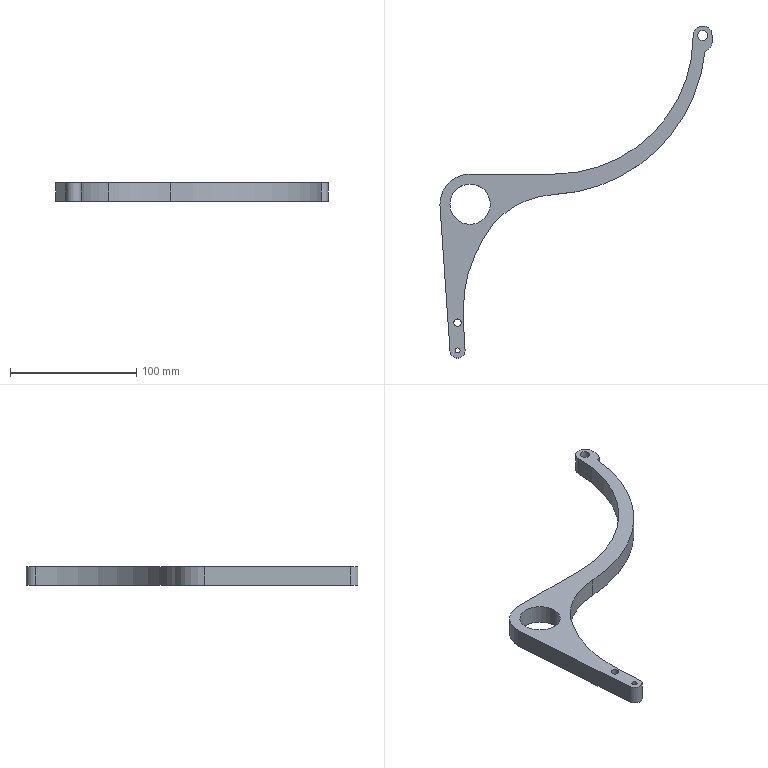Part | SolidWorks | features Extrusion 1 | 1 solid | 21 faces | box 216 x 263.5 x 15 mm | volume 92831 mm3 | cylinder 15 | plane 5 | spline 1 | commonest cylinder face diameters 4 x2 6 x2 7.838 x2 32 x2 12 x1 15 x1
STEP:
#1=CARTESIAN_POINT('',(-3.,22.,15.));
#2=VERTEX_POINT('',#1);
#3=CARTESIAN_POINT('',(3.,22.,15.));
#4=VERTEX_POINT('',#3);
#5=CARTESIAN_POINT('',(0.,22.,15.));
#6=DIRECTION('',(0.,0.,1.));
#7=DIRECTION('',(1.,0.,0.));
#8=AXIS2_PLACEMENT_3D('',#5,#6,#7);
#9=CIRCLE('',#8,3.);
#10=EDGE_CURVE('',#2,#4,#9,.T.);
#11=ORIENTED_EDGE('',*,*,#10,.T.);
#12=CARTESIAN_POINT('',(3.,22.,0.));
#13=VERTEX_POINT('',#12);
#14=CARTESIAN_POINT('',(3.,22.,15.));
#15=DIRECTION('',(0.,0.,-1.));
#16=VECTOR('',#15,1000.);
#17=LINE('',#14,#16);
#18=EDGE_CURVE('',#4,#13,#17,.T.);
#19=ORIENTED_EDGE('',*,*,#18,.T.);
#20=CARTESIAN_POINT('',(-3.,22.,0.));
#21=VERTEX_POINT('',#20);
#22=CARTESIAN_POINT('',(0.,22.,0.));
#23=DIRECTION('',(0.,0.,1.));
#24=DIRECTION('',(1.,0.,0.));
#25=AXIS2_PLACEMENT_3D('',#22,#23,#24);
#26=CIRCLE('',#25,3.);
#27=EDGE_CURVE('',#21,#13,#26,.T.);
#28=ORIENTED_EDGE('',*,*,#27,.F.);
#29=CARTESIAN_POINT('',(-3.,22.,15.));
#30=DIRECTION('',(0.,0.,-1.));
#31=VECTOR('',#30,1000.);
#32=LINE('',#29,#31);
#33=EDGE_CURVE('',#2,#21,#32,.T.);
#34=ORIENTED_EDGE('',*,*,#33,.F.);
#35=EDGE_LOOP('',(#11,#19,#28,#34));
#36=FACE_OUTER_BOUND('',#35,.T.);
#37=CARTESIAN_POINT('',(0.,22.,15.));
#38=DIRECTION('',(0.,0.,-1.));
#39=DIRECTION('',(-1.,0.,0.));
#40=AXIS2_PLACEMENT_3D('',#37,#38,#39);
#41=CYLINDRICAL_SURFACE('',#40,3.);
#42=ADVANCED_FACE('',(#36),#41,.F.);
#43=CARTESIAN_POINT('',(190.581,250.,15.));
#44=VERTEX_POINT('',#43);
#45=CARTESIAN_POINT('',(198.419,250.,15.));
#46=VERTEX_POINT('',#45);
#47=CARTESIAN_POINT('',(194.5,250.,15.));
#48=DIRECTION('',(0.,0.,1.));
#49=DIRECTION('',(1.,0.,0.));
#50=AXIS2_PLACEMENT_3D('',#47,#48,#49);
#51=CIRCLE('',#50,3.919);
#52=EDGE_CURVE('',#44,#46,#51,.T.);
#53=ORIENTED_EDGE('',*,*,#52,.T.);
#54=CARTESIAN_POINT('',(198.419,250.,0.));
#55=VERTEX_POINT('',#54);
#56=CARTESIAN_POINT('',(198.419,250.,15.));
#57=DIRECTION('',(0.,0.,-1.));
#58=VECTOR('',#57,1000.);
#59=LINE('',#56,#58);
#60=EDGE_CURVE('',#46,#55,#59,.T.);
#61=ORIENTED_EDGE('',*,*,#60,.T.);
#62=CARTESIAN_POINT('',(190.581,250.,0.));
#63=VERTEX_POINT('',#62);
#64=CARTESIAN_POINT('',(194.5,250.,0.));
#65=DIRECTION('',(0.,0.,1.));
#66=DIRECTION('',(1.,0.,0.));
#67=AXIS2_PLACEMENT_3D('',#64,#65,#66);
#68=CIRCLE('',#67,3.919);
#69=EDGE_CURVE('',#63,#55,#68,.T.);
#70=ORIENTED_EDGE('',*,*,#69,.F.);
#71=CARTESIAN_POINT('',(190.581,250.,15.));
#72=DIRECTION('',(0.,0.,-1.));
#73=VECTOR('',#72,1000.);
#74=LINE('',#71,#73);
#75=EDGE_CURVE('',#44,#63,#74,.T.);
#76=ORIENTED_EDGE('',*,*,#75,.F.);
#77=EDGE_LOOP('',(#53,#61,#70,#76));
#78=FACE_OUTER_BOUND('',#77,.T.);
#79=CARTESIAN_POINT('',(194.5,250.,15.));
#80=DIRECTION('',(0.,0.,-1.));
#81=DIRECTION('',(-1.,0.,0.));
#82=AXIS2_PLACEMENT_3D('',#79,#80,#81);
#83=CYLINDRICAL_SURFACE('',#82,3.919);
#84=ADVANCED_FACE('',(#78),#83,.F.);
#85=CARTESIAN_POINT('',(-6.,116.,15.));
#86=VERTEX_POINT('',#85);
#87=CARTESIAN_POINT('',(26.,116.,15.));
#88=VERTEX_POINT('',#87);
#89=CARTESIAN_POINT('',(10.,116.,15.));
#90=DIRECTION('',(0.,0.,1.));
#91=DIRECTION('',(1.,0.,0.));
#92=AXIS2_PLACEMENT_3D('',#89,#90,#91);
#93=CIRCLE('',#92,16.);
#94=EDGE_CURVE('',#86,#88,#93,.T.);
#95=ORIENTED_EDGE('',*,*,#94,.T.);
#96=CARTESIAN_POINT('',(26.,116.,0.));
#97=VERTEX_POINT('',#96);
#98=CARTESIAN_POINT('',(26.,116.,15.));
#99=DIRECTION('',(0.,0.,-1.));
#100=VECTOR('',#99,1000.);
#101=LINE('',#98,#100);
#102=EDGE_CURVE('',#88,#97,#101,.T.);
#103=ORIENTED_EDGE('',*,*,#102,.T.);
#104=CARTESIAN_POINT('',(-6.,116.,0.));
#105=VERTEX_POINT('',#104);
#106=CARTESIAN_POINT('',(10.,116.,0.));
#107=DIRECTION('',(0.,0.,1.));
#108=DIRECTION('',(1.,0.,0.));
#109=AXIS2_PLACEMENT_3D('',#106,#107,#108);
#110=CIRCLE('',#109,16.);
#111=EDGE_CURVE('',#105,#97,#110,.T.);
#112=ORIENTED_EDGE('',*,*,#111,.F.);
#113=CARTESIAN_POINT('',(-6.,116.,15.));
#114=DIRECTION('',(0.,0.,-1.));
#115=VECTOR('',#114,1000.);
#116=LINE('',#113,#115);
#117=EDGE_CURVE('',#86,#105,#116,.T.);
#118=ORIENTED_EDGE('',*,*,#117,.F.);
#119=EDGE_LOOP('',(#95,#103,#112,#118));
#120=FACE_OUTER_BOUND('',#119,.T.);
#121=CARTESIAN_POINT('',(10.,116.,15.));
#122=DIRECTION('',(0.,0.,-1.));
#123=DIRECTION('',(-1.,0.,0.));
#124=AXIS2_PLACEMENT_3D('',#121,#122,#123);
#125=CYLINDRICAL_SURFACE('',#124,16.);
#126=ADVANCED_FACE('',(#120),#125,.F.);
#127=CARTESIAN_POINT('',(-2.,0.,15.));
#128=VERTEX_POINT('',#127);
#129=CARTESIAN_POINT('',(2.,0.,15.));
#130=VERTEX_POINT('',#129);
#131=CARTESIAN_POINT('',(0.,0.,15.));
#132=DIRECTION('',(0.,0.,1.));
#133=DIRECTION('',(1.,0.,0.));
#134=AXIS2_PLACEMENT_3D('',#131,#132,#133);
#135=CIRCLE('',#134,2.);
#136=EDGE_CURVE('',#128,#130,#135,.T.);
#137=ORIENTED_EDGE('',*,*,#136,.T.);
#138=CARTESIAN_POINT('',(2.,0.,0.));
#139=VERTEX_POINT('',#138);
#140=CARTESIAN_POINT('',(2.,0.,15.));
#141=DIRECTION('',(0.,0.,-1.));
#142=VECTOR('',#141,1000.);
#143=LINE('',#140,#142);
#144=EDGE_CURVE('',#130,#139,#143,.T.);
#145=ORIENTED_EDGE('',*,*,#144,.T.);
#146=CARTESIAN_POINT('',(-2.,0.,0.));
#147=VERTEX_POINT('',#146);
#148=CARTESIAN_POINT('',(0.,0.,0.));
#149=DIRECTION('',(0.,0.,1.));
#150=DIRECTION('',(1.,0.,0.));
#151=AXIS2_PLACEMENT_3D('',#148,#149,#150);
#152=CIRCLE('',#151,2.);
#153=EDGE_CURVE('',#147,#139,#152,.T.);
#154=ORIENTED_EDGE('',*,*,#153,.F.);
#155=CARTESIAN_POINT('',(-2.,0.,15.));
#156=DIRECTION('',(0.,0.,-1.));
#157=VECTOR('',#156,1000.);
#158=LINE('',#155,#157);
#159=EDGE_CURVE('',#128,#147,#158,.T.);
#160=ORIENTED_EDGE('',*,*,#159,.F.);
#161=EDGE_LOOP('',(#137,#145,#154,#160));
#162=FACE_OUTER_BOUND('',#161,.T.);
#163=CARTESIAN_POINT('',(0.,0.,15.));
#164=DIRECTION('',(0.,0.,-1.));
#165=DIRECTION('',(-1.,0.,0.));
#166=AXIS2_PLACEMENT_3D('',#163,#164,#165);
#167=CYLINDRICAL_SURFACE('',#166,2.);
#168=ADVANCED_FACE('',(#162),#167,.F.);
#169=ORIENTED_EDGE('',*,*,#52,.F.);
#170=CARTESIAN_POINT('',(194.5,250.,15.));
#171=DIRECTION('',(0.,0.,1.));
#172=DIRECTION('',(1.,0.,0.));
#173=AXIS2_PLACEMENT_3D('',#170,#171,#172);
#174=CIRCLE('',#173,3.919);
#175=EDGE_CURVE('',#46,#44,#174,.T.);
#176=ORIENTED_EDGE('',*,*,#175,.F.);
#177=EDGE_LOOP('',(#169,#176));
#178=FACE_BOUND('',#177,.T.);
#179=ORIENTED_EDGE('',*,*,#136,.F.);
#180=CARTESIAN_POINT('',(0.,0.,15.));
#181=DIRECTION('',(0.,0.,1.));
#182=DIRECTION('',(1.,0.,0.));
#183=AXIS2_PLACEMENT_3D('',#180,#181,#182);
#184=CIRCLE('',#183,2.);
#185=EDGE_CURVE('',#130,#128,#184,.T.);
#186=ORIENTED_EDGE('',*,*,#185,.F.);
#187=EDGE_LOOP('',(#179,#186));
#188=FACE_BOUND('',#187,.T.);
#189=CARTESIAN_POINT('',(10.,140.,15.));
#190=VERTEX_POINT('',#189);
#191=CARTESIAN_POINT('',(-14.,116.,15.));
#192=VERTEX_POINT('',#191);
#193=CARTESIAN_POINT('',(10.,116.,15.));
#194=DIRECTION('',(0.,0.,1.));
#195=DIRECTION('',(1.,0.,0.));
#196=AXIS2_PLACEMENT_3D('',#193,#194,#195);
#197=CIRCLE('',#196,24.);
#198=EDGE_CURVE('',#190,#192,#197,.T.);
#199=ORIENTED_EDGE('',*,*,#198,.T.);
#200=CARTESIAN_POINT('',(-6.,0.,15.));
#201=VERTEX_POINT('',#200);
#202=CARTESIAN_POINT('',(-14.,116.,15.));
#203=DIRECTION('',(0.0688,-0.9976,0.));
#204=VECTOR('',#203,1000.);
#205=LINE('',#202,#204);
#206=EDGE_CURVE('',#192,#201,#205,.T.);
#207=ORIENTED_EDGE('',*,*,#206,.T.);
#208=CARTESIAN_POINT('',(6.,0.,15.));
#209=VERTEX_POINT('',#208);
#210=CARTESIAN_POINT('',(0.,0.,15.));
#211=DIRECTION('',(0.,0.,1.));
#212=DIRECTION('',(1.,0.,0.));
#213=AXIS2_PLACEMENT_3D('',#210,#211,#212);
#214=CIRCLE('',#213,6.);
#215=EDGE_CURVE('',#201,#209,#214,.T.);
#216=ORIENTED_EDGE('',*,*,#215,.T.);
#217=CARTESIAN_POINT('',(28.005,100.131,15.));
#218=VERTEX_POINT('',#217);
#219=CARTESIAN_POINT('',(6.,0.,15.));
#220=CARTESIAN_POINT('',(1.589,45.681,15.));
#221=CARTESIAN_POINT('',(5.604,67.643,15.));
#222=CARTESIAN_POINT('',(28.005,100.131,15.));
#223=B_SPLINE_CURVE_WITH_KNOTS('',3,(#219,#220,#221,#222),.UNSPECIFIED.,.F.,.F.,(4,4),(0.,0.7882),.UNSPECIFIED.);
#224=EDGE_CURVE('',#209,#218,#223,.T.);
#225=ORIENTED_EDGE('',*,*,#224,.T.);
#226=CARTESIAN_POINT('',(77.,123.767,15.));
#227=VERTEX_POINT('',#226);
#228=CARTESIAN_POINT('',(80.543,53.825,15.));
#229=DIRECTION('',(0.,0.,-1.));
#230=DIRECTION('',(1.,0.,0.));
#231=AXIS2_PLACEMENT_3D('',#228,#229,#230);
#232=CIRCLE('',#231,70.032);
#233=EDGE_CURVE('',#218,#227,#232,.T.);
#234=ORIENTED_EDGE('',*,*,#233,.T.);
#235=CARTESIAN_POINT('',(196.38,237.495,15.));
#236=VERTEX_POINT('',#235);
#237=CARTESIAN_POINT('',(70.606,250.,15.));
#238=DIRECTION('',(0.,0.,1.));
#239=DIRECTION('',(1.,0.,0.));
#240=AXIS2_PLACEMENT_3D('',#237,#238,#239);
#241=CIRCLE('',#240,126.394);
#242=EDGE_CURVE('',#227,#236,#241,.T.);
#243=ORIENTED_EDGE('',*,*,#242,.T.);
#244=CARTESIAN_POINT('',(202.,245.,15.));
#245=VERTEX_POINT('',#244);
#246=CARTESIAN_POINT('',(194.179,245.,15.));
#247=DIRECTION('',(0.,0.,1.));
#248=DIRECTION('',(1.,0.,0.));
#249=AXIS2_PLACEMENT_3D('',#246,#247,#248);
#250=CIRCLE('',#249,7.821);
#251=EDGE_CURVE('',#236,#245,#250,.T.);
#252=ORIENTED_EDGE('',*,*,#251,.T.);
#253=CARTESIAN_POINT('',(202.,250.,15.));
#254=VERTEX_POINT('',#253);
#255=CARTESIAN_POINT('',(202.,250.,15.));
#256=DIRECTION('',(0.,1.,0.));
#257=VECTOR('',#256,1000.);
#258=LINE('',#255,#257);
#259=EDGE_CURVE('',#245,#254,#258,.T.);
#260=ORIENTED_EDGE('',*,*,#259,.T.);
#261=CARTESIAN_POINT('',(187.,250.,15.));
#262=VERTEX_POINT('',#261);
#263=CARTESIAN_POINT('',(194.5,250.,15.));
#264=DIRECTION('',(0.,0.,1.));
#265=DIRECTION('',(1.,0.,0.));
#266=AXIS2_PLACEMENT_3D('',#263,#264,#265);
#267=CIRCLE('',#266,7.5);
#268=EDGE_CURVE('',#254,#262,#267,.T.);
#269=ORIENTED_EDGE('',*,*,#268,.T.);
#270=CARTESIAN_POINT('',(77.,140.,15.));
#271=VERTEX_POINT('',#270);
#272=CARTESIAN_POINT('',(77.,250.,15.));
#273=DIRECTION('',(0.,0.,-1.));
#274=DIRECTION('',(1.,0.,0.));
#275=AXIS2_PLACEMENT_3D('',#272,#273,#274);
#276=CIRCLE('',#275,110.);
#277=EDGE_CURVE('',#262,#271,#276,.T.);
#278=ORIENTED_EDGE('',*,*,#277,.T.);
#279=CARTESIAN_POINT('',(10.,140.,15.));
#280=DIRECTION('',(-1.,0.,0.));
#281=VECTOR('',#280,1000.);
#282=LINE('',#279,#281);
#283=EDGE_CURVE('',#271,#190,#282,.T.);
#284=ORIENTED_EDGE('',*,*,#283,.T.);
#285=EDGE_LOOP('',(#199,#207,#216,#225,#234,#243,#252,#260,#269,#278,#284));
#286=FACE_OUTER_BOUND('',#285,.T.);
#287=ORIENTED_EDGE('',*,*,#94,.F.);
#288=CARTESIAN_POINT('',(10.,116.,15.));
#289=DIRECTION('',(0.,0.,1.));
#290=DIRECTION('',(1.,0.,0.));
#291=AXIS2_PLACEMENT_3D('',#288,#289,#290);
#292=CIRCLE('',#291,16.);
#293=EDGE_CURVE('',#88,#86,#292,.T.);
#294=ORIENTED_EDGE('',*,*,#293,.F.);
#295=EDGE_LOOP('',(#287,#294));
#296=FACE_BOUND('',#295,.T.);
#297=ORIENTED_EDGE('',*,*,#10,.F.);
#298=CARTESIAN_POINT('',(0.,22.,15.));
#299=DIRECTION('',(0.,0.,1.));
#300=DIRECTION('',(1.,0.,0.));
#301=AXIS2_PLACEMENT_3D('',#298,#299,#300);
#302=CIRCLE('',#301,3.);
#303=EDGE_CURVE('',#4,#2,#302,.T.);
#304=ORIENTED_EDGE('',*,*,#303,.F.);
#305=EDGE_LOOP('',(#297,#304));
#306=FACE_BOUND('',#305,.T.);
#307=CARTESIAN_POINT('',(10.,116.,15.));
#308=DIRECTION('',(0.,0.,1.));
#309=DIRECTION('',(1.,0.,0.));
#310=AXIS2_PLACEMENT_3D('',#307,#308,#309);
#311=PLANE('',#310);
#312=ADVANCED_FACE('',(#178,#188,#286,#296,#306),#311,.T.);
#313=CARTESIAN_POINT('',(10.,140.,0.));
#314=VERTEX_POINT('',#313);
#315=CARTESIAN_POINT('',(-14.,116.,0.));
#316=VERTEX_POINT('',#315);
#317=CARTESIAN_POINT('',(10.,116.,0.));
#318=DIRECTION('',(0.,0.,1.));
#319=DIRECTION('',(1.,0.,0.));
#320=AXIS2_PLACEMENT_3D('',#317,#318,#319);
#321=CIRCLE('',#320,24.);
#322=EDGE_CURVE('',#314,#316,#321,.T.);
#323=ORIENTED_EDGE('',*,*,#322,.F.);
#324=CARTESIAN_POINT('',(77.,140.,0.));
#325=VERTEX_POINT('',#324);
#326=CARTESIAN_POINT('',(10.,140.,0.));
#327=DIRECTION('',(-1.,0.,0.));
#328=VECTOR('',#327,1000.);
#329=LINE('',#326,#328);
#330=EDGE_CURVE('',#325,#314,#329,.T.);
#331=ORIENTED_EDGE('',*,*,#330,.F.);
#332=CARTESIAN_POINT('',(187.,250.,0.));
#333=VERTEX_POINT('',#332);
#334=CARTESIAN_POINT('',(77.,250.,0.));
#335=DIRECTION('',(0.,0.,-1.));
#336=DIRECTION('',(1.,0.,0.));
#337=AXIS2_PLACEMENT_3D('',#334,#335,#336);
#338=CIRCLE('',#337,110.);
#339=EDGE_CURVE('',#333,#325,#338,.T.);
#340=ORIENTED_EDGE('',*,*,#339,.F.);
#341=CARTESIAN_POINT('',(202.,250.,0.));
#342=VERTEX_POINT('',#341);
#343=CARTESIAN_POINT('',(194.5,250.,0.));
#344=DIRECTION('',(0.,0.,1.));
#345=DIRECTION('',(1.,0.,0.));
#346=AXIS2_PLACEMENT_3D('',#343,#344,#345);
#347=CIRCLE('',#346,7.5);
#348=EDGE_CURVE('',#342,#333,#347,.T.);
#349=ORIENTED_EDGE('',*,*,#348,.F.);
#350=CARTESIAN_POINT('',(202.,245.,0.));
#351=VERTEX_POINT('',#350);
#352=CARTESIAN_POINT('',(202.,250.,0.));
#353=DIRECTION('',(0.,1.,0.));
#354=VECTOR('',#353,1000.);
#355=LINE('',#352,#354);
#356=EDGE_CURVE('',#351,#342,#355,.T.);
#357=ORIENTED_EDGE('',*,*,#356,.F.);
#358=CARTESIAN_POINT('',(196.38,237.495,0.));
#359=VERTEX_POINT('',#358);
#360=CARTESIAN_POINT('',(194.179,245.,0.));
#361=DIRECTION('',(0.,0.,1.));
#362=DIRECTION('',(1.,0.,0.));
#363=AXIS2_PLACEMENT_3D('',#360,#361,#362);
#364=CIRCLE('',#363,7.821);
#365=EDGE_CURVE('',#359,#351,#364,.T.);
#366=ORIENTED_EDGE('',*,*,#365,.F.);
#367=CARTESIAN_POINT('',(77.,123.767,0.));
#368=VERTEX_POINT('',#367);
#369=CARTESIAN_POINT('',(70.606,250.,0.));
#370=DIRECTION('',(0.,0.,1.));
#371=DIRECTION('',(1.,0.,0.));
#372=AXIS2_PLACEMENT_3D('',#369,#370,#371);
#373=CIRCLE('',#372,126.394);
#374=EDGE_CURVE('',#368,#359,#373,.T.);
#375=ORIENTED_EDGE('',*,*,#374,.F.);
#376=CARTESIAN_POINT('',(28.005,100.131,0.));
#377=VERTEX_POINT('',#376);
#378=CARTESIAN_POINT('',(80.543,53.825,0.));
#379=DIRECTION('',(0.,0.,-1.));
#380=DIRECTION('',(1.,0.,0.));
#381=AXIS2_PLACEMENT_3D('',#378,#379,#380);
#382=CIRCLE('',#381,70.032);
#383=EDGE_CURVE('',#377,#368,#382,.T.);
#384=ORIENTED_EDGE('',*,*,#383,.F.);
#385=CARTESIAN_POINT('',(6.,0.,0.));
#386=VERTEX_POINT('',#385);
#387=CARTESIAN_POINT('',(6.,0.,0.));
#388=CARTESIAN_POINT('',(1.589,45.681,0.));
#389=CARTESIAN_POINT('',(5.604,67.643,0.));
#390=CARTESIAN_POINT('',(28.005,100.131,0.));
#391=B_SPLINE_CURVE_WITH_KNOTS('',3,(#387,#388,#389,#390),.UNSPECIFIED.,.F.,.F.,(4,4),(0.,0.7882),.UNSPECIFIED.);
#392=EDGE_CURVE('',#386,#377,#391,.T.);
#393=ORIENTED_EDGE('',*,*,#392,.F.);
#394=CARTESIAN_POINT('',(-6.,0.,0.));
#395=VERTEX_POINT('',#394);
#396=CARTESIAN_POINT('',(0.,0.,0.));
#397=DIRECTION('',(0.,0.,1.));
#398=DIRECTION('',(1.,0.,0.));
#399=AXIS2_PLACEMENT_3D('',#396,#397,#398);
#400=CIRCLE('',#399,6.);
#401=EDGE_CURVE('',#395,#386,#400,.T.);
#402=ORIENTED_EDGE('',*,*,#401,.F.);
#403=CARTESIAN_POINT('',(-14.,116.,0.));
#404=DIRECTION('',(0.0688,-0.9976,0.));
#405=VECTOR('',#404,1000.);
#406=LINE('',#403,#405);
#407=EDGE_CURVE('',#316,#395,#406,.T.);
#408=ORIENTED_EDGE('',*,*,#407,.F.);
#409=EDGE_LOOP('',(#323,#331,#340,#349,#357,#366,#375,#384,#393,#402,#408));
#410=FACE_OUTER_BOUND('',#409,.T.);
#411=ORIENTED_EDGE('',*,*,#153,.T.);
#412=CARTESIAN_POINT('',(0.,0.,0.));
#413=DIRECTION('',(0.,0.,1.));
#414=DIRECTION('',(1.,0.,0.));
#415=AXIS2_PLACEMENT_3D('',#412,#413,#414);
#416=CIRCLE('',#415,2.);
#417=EDGE_CURVE('',#139,#147,#416,.T.);
#418=ORIENTED_EDGE('',*,*,#417,.T.);
#419=EDGE_LOOP('',(#411,#418));
#420=FACE_BOUND('',#419,.T.);
#421=ORIENTED_EDGE('',*,*,#111,.T.);
#422=CARTESIAN_POINT('',(10.,116.,0.));
#423=DIRECTION('',(0.,0.,1.));
#424=DIRECTION('',(1.,0.,0.));
#425=AXIS2_PLACEMENT_3D('',#422,#423,#424);
#426=CIRCLE('',#425,16.);
#427=EDGE_CURVE('',#97,#105,#426,.T.);
#428=ORIENTED_EDGE('',*,*,#427,.T.);
#429=EDGE_LOOP('',(#421,#428));
#430=FACE_BOUND('',#429,.T.);
#431=ORIENTED_EDGE('',*,*,#69,.T.);
#432=CARTESIAN_POINT('',(194.5,250.,0.));
#433=DIRECTION('',(0.,0.,1.));
#434=DIRECTION('',(1.,0.,0.));
#435=AXIS2_PLACEMENT_3D('',#432,#433,#434);
#436=CIRCLE('',#435,3.919);
#437=EDGE_CURVE('',#55,#63,#436,.T.);
#438=ORIENTED_EDGE('',*,*,#437,.T.);
#439=EDGE_LOOP('',(#431,#438));
#440=FACE_BOUND('',#439,.T.);
#441=ORIENTED_EDGE('',*,*,#27,.T.);
#442=CARTESIAN_POINT('',(0.,22.,0.));
#443=DIRECTION('',(0.,0.,1.));
#444=DIRECTION('',(1.,0.,0.));
#445=AXIS2_PLACEMENT_3D('',#442,#443,#444);
#446=CIRCLE('',#445,3.);
#447=EDGE_CURVE('',#13,#21,#446,.T.);
#448=ORIENTED_EDGE('',*,*,#447,.T.);
#449=EDGE_LOOP('',(#441,#448));
#450=FACE_BOUND('',#449,.T.);
#451=CARTESIAN_POINT('',(10.,116.,0.));
#452=DIRECTION('',(0.,0.,1.));
#453=DIRECTION('',(1.,0.,0.));
#454=AXIS2_PLACEMENT_3D('',#451,#452,#453);
#455=PLANE('',#454);
#456=ADVANCED_FACE('',(#410,#420,#430,#440,#450),#455,.F.);
#457=ORIENTED_EDGE('',*,*,#322,.T.);
#458=CARTESIAN_POINT('',(-14.,116.,15.));
#459=DIRECTION('',(0.,0.,-1.));
#460=VECTOR('',#459,1000.);
#461=LINE('',#458,#460);
#462=EDGE_CURVE('',#192,#316,#461,.T.);
#463=ORIENTED_EDGE('',*,*,#462,.F.);
#464=ORIENTED_EDGE('',*,*,#198,.F.);
#465=CARTESIAN_POINT('',(10.,140.,15.));
#466=DIRECTION('',(0.,0.,-1.));
#467=VECTOR('',#466,1000.);
#468=LINE('',#465,#467);
#469=EDGE_CURVE('',#190,#314,#468,.T.);
#470=ORIENTED_EDGE('',*,*,#469,.T.);
#471=EDGE_LOOP('',(#457,#463,#464,#470));
#472=FACE_OUTER_BOUND('',#471,.T.);
#473=CARTESIAN_POINT('',(10.,116.,15.));
#474=DIRECTION('',(0.,0.,-1.));
#475=DIRECTION('',(-1.,0.,0.));
#476=AXIS2_PLACEMENT_3D('',#473,#474,#475);
#477=CYLINDRICAL_SURFACE('',#476,24.);
#478=ADVANCED_FACE('',(#472),#477,.T.);
#479=ORIENTED_EDGE('',*,*,#407,.T.);
#480=CARTESIAN_POINT('',(-6.,0.,15.));
#481=DIRECTION('',(0.,0.,-1.));
#482=VECTOR('',#481,1000.);
#483=LINE('',#480,#482);
#484=EDGE_CURVE('',#201,#395,#483,.T.);
#485=ORIENTED_EDGE('',*,*,#484,.F.);
#486=ORIENTED_EDGE('',*,*,#206,.F.);
#487=ORIENTED_EDGE('',*,*,#462,.T.);
#488=EDGE_LOOP('',(#479,#485,#486,#487));
#489=FACE_OUTER_BOUND('',#488,.T.);
#490=CARTESIAN_POINT('',(-14.,116.,15.));
#491=DIRECTION('',(0.9976,0.0688,0.));
#492=DIRECTION('',(-0.0688,0.9976,0.));
#493=AXIS2_PLACEMENT_3D('',#490,#491,#492);
#494=PLANE('',#493);
#495=ADVANCED_FACE('',(#489),#494,.F.);
#496=ORIENTED_EDGE('',*,*,#401,.T.);
#497=CARTESIAN_POINT('',(6.,0.,15.));
#498=DIRECTION('',(0.,0.,-1.));
#499=VECTOR('',#498,1000.);
#500=LINE('',#497,#499);
#501=EDGE_CURVE('',#209,#386,#500,.T.);
#502=ORIENTED_EDGE('',*,*,#501,.F.);
#503=ORIENTED_EDGE('',*,*,#215,.F.);
#504=ORIENTED_EDGE('',*,*,#484,.T.);
#505=EDGE_LOOP('',(#496,#502,#503,#504));
#506=FACE_OUTER_BOUND('',#505,.T.);
#507=CARTESIAN_POINT('',(0.,0.,15.));
#508=DIRECTION('',(0.,0.,-1.));
#509=DIRECTION('',(-1.,0.,0.));
#510=AXIS2_PLACEMENT_3D('',#507,#508,#509);
#511=CYLINDRICAL_SURFACE('',#510,6.);
#512=ADVANCED_FACE('',(#506),#511,.T.);
#513=ORIENTED_EDGE('',*,*,#392,.T.);
#514=CARTESIAN_POINT('',(28.005,100.131,15.));
#515=DIRECTION('',(0.,0.,-1.));
#516=VECTOR('',#515,1000.);
#517=LINE('',#514,#516);
#518=EDGE_CURVE('',#218,#377,#517,.T.);
#519=ORIENTED_EDGE('',*,*,#518,.F.);
#520=ORIENTED_EDGE('',*,*,#224,.F.);
#521=ORIENTED_EDGE('',*,*,#501,.T.);
#522=EDGE_LOOP('',(#513,#519,#520,#521));
#523=FACE_OUTER_BOUND('',#522,.T.);
#524=CARTESIAN_POINT('',(6.,0.,15.));
#525=CARTESIAN_POINT('',(6.,0.,0.));
#526=CARTESIAN_POINT('',(1.589,45.681,15.));
#527=CARTESIAN_POINT('',(1.589,45.681,0.));
#528=CARTESIAN_POINT('',(5.604,67.643,15.));
#529=CARTESIAN_POINT('',(5.604,67.643,0.));
#530=CARTESIAN_POINT('',(28.005,100.131,15.));
#531=CARTESIAN_POINT('',(28.005,100.131,0.));
#532=B_SPLINE_SURFACE_WITH_KNOTS('',3,1,((#524,#525),(#526,#527),(#528,#529),(#530,#531)),.UNSPECIFIED.,.F.,.F.,.F.,(4,4),(2,2),(0.,0.7882),(0.,1.),.UNSPECIFIED.);
#533=ADVANCED_FACE('',(#523),#532,.F.);
#534=ORIENTED_EDGE('',*,*,#383,.T.);
#535=CARTESIAN_POINT('',(77.,123.767,15.));
#536=DIRECTION('',(0.,0.,-1.));
#537=VECTOR('',#536,1000.);
#538=LINE('',#535,#537);
#539=EDGE_CURVE('',#227,#368,#538,.T.);
#540=ORIENTED_EDGE('',*,*,#539,.F.);
#541=ORIENTED_EDGE('',*,*,#233,.F.);
#542=ORIENTED_EDGE('',*,*,#518,.T.);
#543=EDGE_LOOP('',(#534,#540,#541,#542));
#544=FACE_OUTER_BOUND('',#543,.T.);
#545=CARTESIAN_POINT('',(80.543,53.825,15.));
#546=DIRECTION('',(0.,0.,-1.));
#547=DIRECTION('',(-1.,0.,0.));
#548=AXIS2_PLACEMENT_3D('',#545,#546,#547);
#549=CYLINDRICAL_SURFACE('',#548,70.032);
#550=ADVANCED_FACE('',(#544),#549,.F.);
#551=ORIENTED_EDGE('',*,*,#374,.T.);
#552=CARTESIAN_POINT('',(196.38,237.495,15.));
#553=DIRECTION('',(0.,0.,-1.));
#554=VECTOR('',#553,1000.);
#555=LINE('',#552,#554);
#556=EDGE_CURVE('',#236,#359,#555,.T.);
#557=ORIENTED_EDGE('',*,*,#556,.F.);
#558=ORIENTED_EDGE('',*,*,#242,.F.);
#559=ORIENTED_EDGE('',*,*,#539,.T.);
#560=EDGE_LOOP('',(#551,#557,#558,#559));
#561=FACE_OUTER_BOUND('',#560,.T.);
#562=CARTESIAN_POINT('',(70.606,250.,15.));
#563=DIRECTION('',(0.,0.,-1.));
#564=DIRECTION('',(-1.,0.,0.));
#565=AXIS2_PLACEMENT_3D('',#562,#563,#564);
#566=CYLINDRICAL_SURFACE('',#565,126.394);
#567=ADVANCED_FACE('',(#561),#566,.T.);
#568=ORIENTED_EDGE('',*,*,#365,.T.);
#569=CARTESIAN_POINT('',(202.,245.,15.));
#570=DIRECTION('',(0.,0.,-1.));
#571=VECTOR('',#570,1000.);
#572=LINE('',#569,#571);
#573=EDGE_CURVE('',#245,#351,#572,.T.);
#574=ORIENTED_EDGE('',*,*,#573,.F.);
#575=ORIENTED_EDGE('',*,*,#251,.F.);
#576=ORIENTED_EDGE('',*,*,#556,.T.);
#577=EDGE_LOOP('',(#568,#574,#575,#576));
#578=FACE_OUTER_BOUND('',#577,.T.);
#579=CARTESIAN_POINT('',(194.179,245.,15.));
#580=DIRECTION('',(0.,0.,-1.));
#581=DIRECTION('',(-1.,0.,0.));
#582=AXIS2_PLACEMENT_3D('',#579,#580,#581);
#583=CYLINDRICAL_SURFACE('',#582,7.821);
#584=ADVANCED_FACE('',(#578),#583,.T.);
#585=ORIENTED_EDGE('',*,*,#356,.T.);
#586=CARTESIAN_POINT('',(202.,250.,15.));
#587=DIRECTION('',(0.,0.,-1.));
#588=VECTOR('',#587,1000.);
#589=LINE('',#586,#588);
#590=EDGE_CURVE('',#254,#342,#589,.T.);
#591=ORIENTED_EDGE('',*,*,#590,.F.);
#592=ORIENTED_EDGE('',*,*,#259,.F.);
#593=ORIENTED_EDGE('',*,*,#573,.T.);
#594=EDGE_LOOP('',(#585,#591,#592,#593));
#595=FACE_OUTER_BOUND('',#594,.T.);
#596=CARTESIAN_POINT('',(202.,250.,15.));
#597=DIRECTION('',(-1.,0.,0.));
#598=DIRECTION('',(0.,0.,1.));
#599=AXIS2_PLACEMENT_3D('',#596,#597,#598);
#600=PLANE('',#599);
#601=ADVANCED_FACE('',(#595),#600,.F.);
#602=ORIENTED_EDGE('',*,*,#348,.T.);
#603=CARTESIAN_POINT('',(187.,250.,15.));
#604=DIRECTION('',(0.,0.,-1.));
#605=VECTOR('',#604,1000.);
#606=LINE('',#603,#605);
#607=EDGE_CURVE('',#262,#333,#606,.T.);
#608=ORIENTED_EDGE('',*,*,#607,.F.);
#609=ORIENTED_EDGE('',*,*,#268,.F.);
#610=ORIENTED_EDGE('',*,*,#590,.T.);
#611=EDGE_LOOP('',(#602,#608,#609,#610));
#612=FACE_OUTER_BOUND('',#611,.T.);
#613=CARTESIAN_POINT('',(194.5,250.,15.));
#614=DIRECTION('',(0.,0.,-1.));
#615=DIRECTION('',(-1.,0.,0.));
#616=AXIS2_PLACEMENT_3D('',#613,#614,#615);
#617=CYLINDRICAL_SURFACE('',#616,7.5);
#618=ADVANCED_FACE('',(#612),#617,.T.);
#619=ORIENTED_EDGE('',*,*,#339,.T.);
#620=CARTESIAN_POINT('',(77.,140.,15.));
#621=DIRECTION('',(0.,0.,-1.));
#622=VECTOR('',#621,1000.);
#623=LINE('',#620,#622);
#624=EDGE_CURVE('',#271,#325,#623,.T.);
#625=ORIENTED_EDGE('',*,*,#624,.F.);
#626=ORIENTED_EDGE('',*,*,#277,.F.);
#627=ORIENTED_EDGE('',*,*,#607,.T.);
#628=EDGE_LOOP('',(#619,#625,#626,#627));
#629=FACE_OUTER_BOUND('',#628,.T.);
#630=CARTESIAN_POINT('',(77.,250.,15.));
#631=DIRECTION('',(0.,0.,-1.));
#632=DIRECTION('',(-1.,0.,0.));
#633=AXIS2_PLACEMENT_3D('',#630,#631,#632);
#634=CYLINDRICAL_SURFACE('',#633,110.);
#635=ADVANCED_FACE('',(#629),#634,.F.);
#636=ORIENTED_EDGE('',*,*,#330,.T.);
#637=ORIENTED_EDGE('',*,*,#469,.F.);
#638=ORIENTED_EDGE('',*,*,#283,.F.);
#639=ORIENTED_EDGE('',*,*,#624,.T.);
#640=EDGE_LOOP('',(#636,#637,#638,#639));
#641=FACE_OUTER_BOUND('',#640,.T.);
#642=CARTESIAN_POINT('',(10.,140.,15.));
#643=DIRECTION('',(0.,-1.,0.));
#644=DIRECTION('',(0.,0.,-1.));
#645=AXIS2_PLACEMENT_3D('',#642,#643,#644);
#646=PLANE('',#645);
#647=ADVANCED_FACE('',(#641),#646,.F.);
#648=ORIENTED_EDGE('',*,*,#144,.F.);
#649=ORIENTED_EDGE('',*,*,#185,.T.);
#650=ORIENTED_EDGE('',*,*,#159,.T.);
#651=ORIENTED_EDGE('',*,*,#417,.F.);
#652=EDGE_LOOP('',(#648,#649,#650,#651));
#653=FACE_OUTER_BOUND('',#652,.T.);
#654=CARTESIAN_POINT('',(0.,0.,15.));
#655=DIRECTION('',(0.,0.,-1.));
#656=DIRECTION('',(-1.,0.,0.));
#657=AXIS2_PLACEMENT_3D('',#654,#655,#656);
#658=CYLINDRICAL_SURFACE('',#657,2.);
#659=ADVANCED_FACE('',(#653),#658,.F.);
#660=ORIENTED_EDGE('',*,*,#102,.F.);
#661=ORIENTED_EDGE('',*,*,#293,.T.);
#662=ORIENTED_EDGE('',*,*,#117,.T.);
#663=ORIENTED_EDGE('',*,*,#427,.F.);
#664=EDGE_LOOP('',(#660,#661,#662,#663));
#665=FACE_OUTER_BOUND('',#664,.T.);
#666=CARTESIAN_POINT('',(10.,116.,15.));
#667=DIRECTION('',(0.,0.,-1.));
#668=DIRECTION('',(-1.,0.,0.));
#669=AXIS2_PLACEMENT_3D('',#666,#667,#668);
#670=CYLINDRICAL_SURFACE('',#669,16.);
#671=ADVANCED_FACE('',(#665),#670,.F.);
#672=ORIENTED_EDGE('',*,*,#60,.F.);
#673=ORIENTED_EDGE('',*,*,#175,.T.);
#674=ORIENTED_EDGE('',*,*,#75,.T.);
#675=ORIENTED_EDGE('',*,*,#437,.F.);
#676=EDGE_LOOP('',(#672,#673,#674,#675));
#677=FACE_OUTER_BOUND('',#676,.T.);
#678=CARTESIAN_POINT('',(194.5,250.,15.));
#679=DIRECTION('',(0.,0.,-1.));
#680=DIRECTION('',(-1.,0.,0.));
#681=AXIS2_PLACEMENT_3D('',#678,#679,#680);
#682=CYLINDRICAL_SURFACE('',#681,3.919);
#683=ADVANCED_FACE('',(#677),#682,.F.);
#684=ORIENTED_EDGE('',*,*,#18,.F.);
#685=ORIENTED_EDGE('',*,*,#303,.T.);
#686=ORIENTED_EDGE('',*,*,#33,.T.);
#687=ORIENTED_EDGE('',*,*,#447,.F.);
#688=EDGE_LOOP('',(#684,#685,#686,#687));
#689=FACE_OUTER_BOUND('',#688,.T.);
#690=CARTESIAN_POINT('',(0.,22.,15.));
#691=DIRECTION('',(0.,0.,-1.));
#692=DIRECTION('',(-1.,0.,0.));
#693=AXIS2_PLACEMENT_3D('',#690,#691,#692);
#694=CYLINDRICAL_SURFACE('',#693,3.);
#695=ADVANCED_FACE('',(#689),#694,.F.);
#696=CLOSED_SHELL('',(#42,#84,#126,#168,#312,#456,#478,#495,#512,#533,#550,#567,#584,#601,#618,#635,#647,#659,#671,#683,#695));
#697=MANIFOLD_SOLID_BREP('',#696);
#698=CARTESIAN_POINT('',(0.,0.,0.));
#699=DIRECTION('',(0.,0.,1.));
#700=DIRECTION('',(1.,0.,0.));
#701=AXIS2_PLACEMENT_3D('',#698,#699,#700);
#702=(LENGTH_UNIT()NAMED_UNIT(*)SI_UNIT(.MILLI.,.METRE.));
#703=UNCERTAINTY_MEASURE_WITH_UNIT(LENGTH_MEASURE(0.00001),#702,'','');
#704=(NAMED_UNIT(*)PLANE_ANGLE_UNIT()SI_UNIT($,.RADIAN.));
#705=(NAMED_UNIT(*)SI_UNIT($,.STERADIAN.)SOLID_ANGLE_UNIT());
#706=(GEOMETRIC_REPRESENTATION_CONTEXT(3)GLOBAL_UNCERTAINTY_ASSIGNED_CONTEXT((#703))GLOBAL_UNIT_ASSIGNED_CONTEXT((#702,#704,#705))REPRESENTATION_CONTEXT('',''));
#707=ADVANCED_BREP_SHAPE_REPRESENTATION('',(#697,#701),#706);